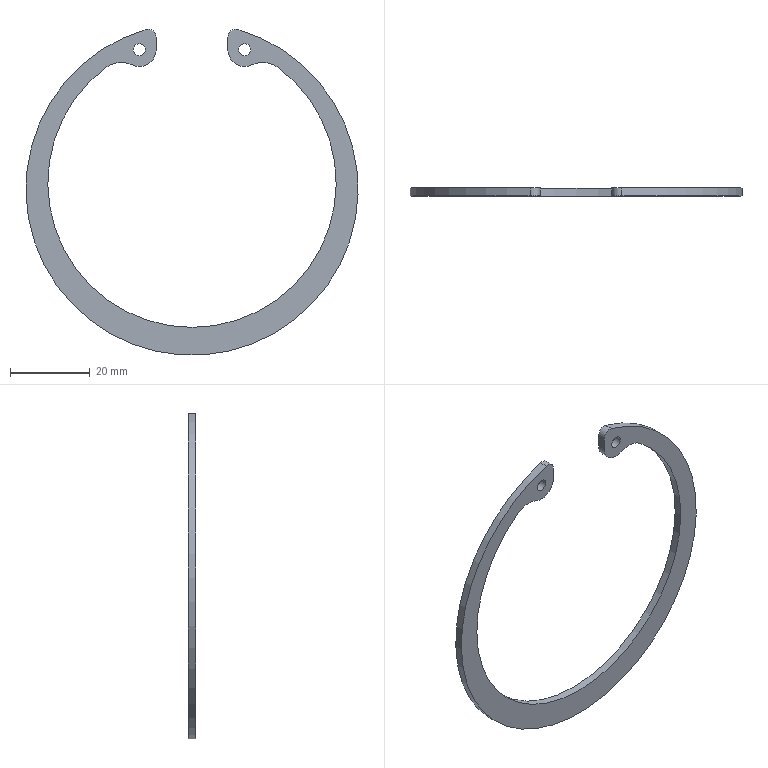Part | STEP file | Ring A80.65Г GOST 13943-86 | 1 solid | 14 faces | box 83.5 x 2 x 81.948 mm | volume 2646 mm3 | cylinder 10 | plane 4 | commonest cylinder face diameters 3 x2 4 x2 8.5 x2 13 x2 72.5 x1 83.5 x1
STEP:
#1=CARTESIAN_POINT('',(-21.685,0.,29.049));
#2=VERTEX_POINT('',#1);
#3=CARTESIAN_POINT('',(-21.685,2.,29.049));
#4=VERTEX_POINT('',#3);
#5=CARTESIAN_POINT('',(-21.685,0.,29.049));
#6=DIRECTION('',(0.,1.,0.));
#7=VECTOR('',#6,1.);
#8=LINE('',#5,#7);
#9=EDGE_CURVE('',#2,#4,#8,.T.);
#10=ORIENTED_EDGE('',*,*,#9,.F.);
#11=CARTESIAN_POINT('',(21.685,0.,29.049));
#12=VERTEX_POINT('',#11);
#13=CARTESIAN_POINT('',(0.,0.,0.));
#14=DIRECTION('',(0.,1.,0.));
#15=DIRECTION('',(0.5982,0.,0.8013));
#16=AXIS2_PLACEMENT_3D('',#13,#14,#15);
#17=CIRCLE('',#16,36.25);
#18=EDGE_CURVE('',#12,#2,#17,.T.);
#19=ORIENTED_EDGE('',*,*,#18,.F.);
#20=CARTESIAN_POINT('',(21.685,2.,29.049));
#21=VERTEX_POINT('',#20);
#22=CARTESIAN_POINT('',(21.685,0.,29.049));
#23=DIRECTION('',(0.,1.,0.));
#24=VECTOR('',#23,1.);
#25=LINE('',#22,#24);
#26=EDGE_CURVE('',#12,#21,#25,.T.);
#27=ORIENTED_EDGE('',*,*,#26,.T.);
#28=CARTESIAN_POINT('',(0.,2.,0.));
#29=DIRECTION('',(0.,1.,0.));
#30=DIRECTION('',(0.5982,0.,0.8013));
#31=AXIS2_PLACEMENT_3D('',#28,#29,#30);
#32=CIRCLE('',#31,36.25);
#33=EDGE_CURVE('',#4,#21,#32,.F.);
#34=ORIENTED_EDGE('',*,*,#33,.F.);
#35=EDGE_LOOP('',(#10,#19,#27,#34));
#36=FACE_BOUND('',#35,.T.);
#37=CARTESIAN_POINT('',(0.,0.,0.));
#38=DIRECTION('',(0.,1.,0.));
#39=DIRECTION('',(0.,0.,-1.));
#40=AXIS2_PLACEMENT_3D('',#37,#38,#39);
#41=CYLINDRICAL_SURFACE('',#40,36.25);
#42=ADVANCED_FACE('',(#36),#41,.F.);
#43=CARTESIAN_POINT('',(11.553,2.,38.62));
#44=VERTEX_POINT('',#43);
#45=CARTESIAN_POINT('',(11.553,0.,38.62));
#46=VERTEX_POINT('',#45);
#47=CARTESIAN_POINT('',(11.553,0.,38.62));
#48=DIRECTION('',(0.,1.,0.));
#49=VECTOR('',#48,1.);
#50=LINE('',#47,#49);
#51=EDGE_CURVE('',#44,#46,#50,.F.);
#52=ORIENTED_EDGE('',*,*,#51,.T.);
#53=CARTESIAN_POINT('',(-11.553,0.,38.62));
#54=VERTEX_POINT('',#53);
#55=CARTESIAN_POINT('',(0.,0.,-1.5));
#56=DIRECTION('',(0.,1.,0.));
#57=DIRECTION('',(0.2767,0.,0.9609));
#58=AXIS2_PLACEMENT_3D('',#55,#56,#57);
#59=CIRCLE('',#58,41.75);
#60=EDGE_CURVE('',#46,#54,#59,.T.);
#61=ORIENTED_EDGE('',*,*,#60,.T.);
#62=CARTESIAN_POINT('',(-11.553,2.,38.62));
#63=VERTEX_POINT('',#62);
#64=CARTESIAN_POINT('',(-11.553,0.,38.62));
#65=DIRECTION('',(0.,1.,0.));
#66=VECTOR('',#65,1.);
#67=LINE('',#64,#66);
#68=EDGE_CURVE('',#54,#63,#67,.T.);
#69=ORIENTED_EDGE('',*,*,#68,.T.);
#70=CARTESIAN_POINT('',(0.,2.,-1.5));
#71=DIRECTION('',(0.,1.,0.));
#72=DIRECTION('',(0.2767,0.,0.9609));
#73=AXIS2_PLACEMENT_3D('',#70,#71,#72);
#74=CIRCLE('',#73,41.75);
#75=EDGE_CURVE('',#44,#63,#74,.T.);
#76=ORIENTED_EDGE('',*,*,#75,.F.);
#77=EDGE_LOOP('',(#52,#61,#69,#76));
#78=FACE_BOUND('',#77,.T.);
#79=CARTESIAN_POINT('',(0.,0.,-1.5));
#80=DIRECTION('',(0.,1.,0.));
#81=DIRECTION('',(1.,0.,0.));
#82=AXIS2_PLACEMENT_3D('',#79,#80,#81);
#83=CYLINDRICAL_SURFACE('',#82,41.75);
#84=ADVANCED_FACE('',(#78),#83,.T.);
#85=CARTESIAN_POINT('',(9.,2.,36.698));
#86=VERTEX_POINT('',#85);
#87=CARTESIAN_POINT('',(11.,2.,36.698));
#88=DIRECTION('',(0.,-1.,0.));
#89=DIRECTION('',(0.2767,0.,0.9609));
#90=AXIS2_PLACEMENT_3D('',#87,#88,#89);
#91=CIRCLE('',#90,2.);
#92=EDGE_CURVE('',#44,#86,#91,.T.);
#93=ORIENTED_EDGE('',*,*,#92,.F.);
#94=ORIENTED_EDGE('',*,*,#75,.T.);
#95=CARTESIAN_POINT('',(-9.,2.,36.698));
#96=VERTEX_POINT('',#95);
#97=CARTESIAN_POINT('',(-11.,2.,36.698));
#98=DIRECTION('',(0.,-1.,0.));
#99=DIRECTION('',(1.,0.,0.));
#100=AXIS2_PLACEMENT_3D('',#97,#98,#99);
#101=CIRCLE('',#100,2.);
#102=EDGE_CURVE('',#96,#63,#101,.T.);
#103=ORIENTED_EDGE('',*,*,#102,.F.);
#104=CARTESIAN_POINT('',(-9.,2.,33.581));
#105=VERTEX_POINT('',#104);
#106=CARTESIAN_POINT('',(-9.,2.,33.581));
#107=DIRECTION('',(0.,0.,1.));
#108=VECTOR('',#107,1.);
#109=LINE('',#106,#108);
#110=EDGE_CURVE('',#96,#105,#109,.F.);
#111=ORIENTED_EDGE('',*,*,#110,.T.);
#112=CARTESIAN_POINT('',(-15.047,2.,29.73));
#113=VERTEX_POINT('',#112);
#114=CARTESIAN_POINT('',(-13.25,2.,33.581));
#115=DIRECTION('',(0.,-1.,0.));
#116=DIRECTION('',(-0.4229,0.,-0.9062));
#117=AXIS2_PLACEMENT_3D('',#114,#115,#116);
#118=CIRCLE('',#117,4.25);
#119=EDGE_CURVE('',#105,#113,#118,.F.);
#120=ORIENTED_EDGE('',*,*,#119,.T.);
#121=CARTESIAN_POINT('',(-17.797,2.,23.84));
#122=DIRECTION('',(0.,1.,0.));
#123=DIRECTION('',(-0.5982,0.,0.8013));
#124=AXIS2_PLACEMENT_3D('',#121,#122,#123);
#125=CIRCLE('',#124,6.5);
#126=EDGE_CURVE('',#113,#4,#125,.F.);
#127=ORIENTED_EDGE('',*,*,#126,.T.);
#128=ORIENTED_EDGE('',*,*,#33,.T.);
#129=CARTESIAN_POINT('',(15.047,2.,29.73));
#130=VERTEX_POINT('',#129);
#131=CARTESIAN_POINT('',(17.797,2.,23.84));
#132=DIRECTION('',(0.,1.,0.));
#133=DIRECTION('',(-0.4229,0.,0.9062));
#134=AXIS2_PLACEMENT_3D('',#131,#132,#133);
#135=CIRCLE('',#134,6.5);
#136=EDGE_CURVE('',#21,#130,#135,.F.);
#137=ORIENTED_EDGE('',*,*,#136,.T.);
#138=CARTESIAN_POINT('',(9.,2.,33.581));
#139=VERTEX_POINT('',#138);
#140=CARTESIAN_POINT('',(13.25,2.,33.581));
#141=DIRECTION('',(0.,-1.,0.));
#142=DIRECTION('',(-1.,0.,0.));
#143=AXIS2_PLACEMENT_3D('',#140,#141,#142);
#144=CIRCLE('',#143,4.25);
#145=EDGE_CURVE('',#130,#139,#144,.F.);
#146=ORIENTED_EDGE('',*,*,#145,.T.);
#147=CARTESIAN_POINT('',(9.,2.,36.698));
#148=DIRECTION('',(0.,0.,-1.));
#149=VECTOR('',#148,1.);
#150=LINE('',#147,#149);
#151=EDGE_CURVE('',#139,#86,#150,.F.);
#152=ORIENTED_EDGE('',*,*,#151,.T.);
#153=EDGE_LOOP('',(#93,#94,#103,#111,#120,#127,#128,#137,#146,#152));
#154=FACE_BOUND('',#153,.T.);
#155=CARTESIAN_POINT('',(-11.75,2.,33.581));
#156=VERTEX_POINT('',#155);
#157=CARTESIAN_POINT('',(-13.25,2.,33.581));
#158=DIRECTION('',(0.,1.,0.));
#159=DIRECTION('',(1.,0.,0.));
#160=AXIS2_PLACEMENT_3D('',#157,#158,#159);
#161=CIRCLE('',#160,1.5);
#162=EDGE_CURVE('',#156,#156,#161,.F.);
#163=ORIENTED_EDGE('',*,*,#162,.T.);
#164=EDGE_LOOP('',(#163));
#165=FACE_BOUND('',#164,.T.);
#166=CARTESIAN_POINT('',(11.75,2.,33.581));
#167=VERTEX_POINT('',#166);
#168=CARTESIAN_POINT('',(13.25,2.,33.581));
#169=DIRECTION('',(0.,1.,0.));
#170=DIRECTION('',(-1.,0.,0.));
#171=AXIS2_PLACEMENT_3D('',#168,#169,#170);
#172=CIRCLE('',#171,1.5);
#173=EDGE_CURVE('',#167,#167,#172,.F.);
#174=ORIENTED_EDGE('',*,*,#173,.T.);
#175=EDGE_LOOP('',(#174));
#176=FACE_BOUND('',#175,.T.);
#177=CARTESIAN_POINT('',(0.,2.,0.));
#178=DIRECTION('',(0.,1.,0.));
#179=DIRECTION('',(1.,0.,0.));
#180=AXIS2_PLACEMENT_3D('',#177,#178,#179);
#181=PLANE('',#180);
#182=ADVANCED_FACE('',(#154,#165,#176),#181,.T.);
#183=CARTESIAN_POINT('',(9.,0.,36.698));
#184=VERTEX_POINT('',#183);
#185=CARTESIAN_POINT('',(11.,0.,36.698));
#186=DIRECTION('',(0.,-1.,0.));
#187=DIRECTION('',(0.2767,0.,0.9609));
#188=AXIS2_PLACEMENT_3D('',#185,#186,#187);
#189=CIRCLE('',#188,2.);
#190=EDGE_CURVE('',#184,#46,#189,.F.);
#191=ORIENTED_EDGE('',*,*,#190,.F.);
#192=CARTESIAN_POINT('',(9.,0.,33.581));
#193=VERTEX_POINT('',#192);
#194=CARTESIAN_POINT('',(9.,0.,36.698));
#195=DIRECTION('',(0.,0.,-1.));
#196=VECTOR('',#195,1.);
#197=LINE('',#194,#196);
#198=EDGE_CURVE('',#184,#193,#197,.T.);
#199=ORIENTED_EDGE('',*,*,#198,.T.);
#200=CARTESIAN_POINT('',(15.047,0.,29.73));
#201=VERTEX_POINT('',#200);
#202=CARTESIAN_POINT('',(13.25,0.,33.581));
#203=DIRECTION('',(0.,-1.,0.));
#204=DIRECTION('',(-1.,0.,0.));
#205=AXIS2_PLACEMENT_3D('',#202,#203,#204);
#206=CIRCLE('',#205,4.25);
#207=EDGE_CURVE('',#193,#201,#206,.T.);
#208=ORIENTED_EDGE('',*,*,#207,.T.);
#209=CARTESIAN_POINT('',(17.797,0.,23.84));
#210=DIRECTION('',(0.,1.,0.));
#211=DIRECTION('',(-0.4229,0.,0.9062));
#212=AXIS2_PLACEMENT_3D('',#209,#210,#211);
#213=CIRCLE('',#212,6.5);
#214=EDGE_CURVE('',#201,#12,#213,.T.);
#215=ORIENTED_EDGE('',*,*,#214,.T.);
#216=ORIENTED_EDGE('',*,*,#18,.T.);
#217=CARTESIAN_POINT('',(-15.047,0.,29.73));
#218=VERTEX_POINT('',#217);
#219=CARTESIAN_POINT('',(-17.797,0.,23.84));
#220=DIRECTION('',(0.,1.,0.));
#221=DIRECTION('',(-0.5982,0.,0.8013));
#222=AXIS2_PLACEMENT_3D('',#219,#220,#221);
#223=CIRCLE('',#222,6.5);
#224=EDGE_CURVE('',#2,#218,#223,.T.);
#225=ORIENTED_EDGE('',*,*,#224,.T.);
#226=CARTESIAN_POINT('',(-9.,0.,33.581));
#227=VERTEX_POINT('',#226);
#228=CARTESIAN_POINT('',(-13.25,0.,33.581));
#229=DIRECTION('',(0.,-1.,0.));
#230=DIRECTION('',(-0.4229,0.,-0.9062));
#231=AXIS2_PLACEMENT_3D('',#228,#229,#230);
#232=CIRCLE('',#231,4.25);
#233=EDGE_CURVE('',#218,#227,#232,.T.);
#234=ORIENTED_EDGE('',*,*,#233,.T.);
#235=CARTESIAN_POINT('',(-9.,0.,36.698));
#236=VERTEX_POINT('',#235);
#237=CARTESIAN_POINT('',(-9.,0.,33.581));
#238=DIRECTION('',(0.,0.,1.));
#239=VECTOR('',#238,1.);
#240=LINE('',#237,#239);
#241=EDGE_CURVE('',#227,#236,#240,.T.);
#242=ORIENTED_EDGE('',*,*,#241,.T.);
#243=CARTESIAN_POINT('',(-11.,0.,36.698));
#244=DIRECTION('',(0.,-1.,0.));
#245=DIRECTION('',(1.,0.,0.));
#246=AXIS2_PLACEMENT_3D('',#243,#244,#245);
#247=CIRCLE('',#246,2.);
#248=EDGE_CURVE('',#54,#236,#247,.F.);
#249=ORIENTED_EDGE('',*,*,#248,.F.);
#250=ORIENTED_EDGE('',*,*,#60,.F.);
#251=EDGE_LOOP('',(#191,#199,#208,#215,#216,#225,#234,#242,#249,#250));
#252=FACE_BOUND('',#251,.T.);
#253=CARTESIAN_POINT('',(-11.75,0.,33.581));
#254=VERTEX_POINT('',#253);
#255=CARTESIAN_POINT('',(-13.25,0.,33.581));
#256=DIRECTION('',(0.,1.,0.));
#257=DIRECTION('',(1.,0.,0.));
#258=AXIS2_PLACEMENT_3D('',#255,#256,#257);
#259=CIRCLE('',#258,1.5);
#260=EDGE_CURVE('',#254,#254,#259,.T.);
#261=ORIENTED_EDGE('',*,*,#260,.T.);
#262=EDGE_LOOP('',(#261));
#263=FACE_BOUND('',#262,.T.);
#264=CARTESIAN_POINT('',(11.75,0.,33.581));
#265=VERTEX_POINT('',#264);
#266=CARTESIAN_POINT('',(13.25,0.,33.581));
#267=DIRECTION('',(0.,1.,0.));
#268=DIRECTION('',(-1.,0.,0.));
#269=AXIS2_PLACEMENT_3D('',#266,#267,#268);
#270=CIRCLE('',#269,1.5);
#271=EDGE_CURVE('',#265,#265,#270,.T.);
#272=ORIENTED_EDGE('',*,*,#271,.T.);
#273=EDGE_LOOP('',(#272));
#274=FACE_BOUND('',#273,.T.);
#275=CARTESIAN_POINT('',(0.,0.,0.));
#276=DIRECTION('',(0.,1.,0.));
#277=DIRECTION('',(1.,0.,0.));
#278=AXIS2_PLACEMENT_3D('',#275,#276,#277);
#279=PLANE('',#278);
#280=ADVANCED_FACE('',(#252,#263,#274),#279,.F.);
#281=ORIENTED_EDGE('',*,*,#173,.F.);
#282=EDGE_LOOP('',(#281));
#283=FACE_OUTER_BOUND('',#282,.T.);
#284=ORIENTED_EDGE('',*,*,#271,.F.);
#285=EDGE_LOOP('',(#284));
#286=FACE_OUTER_BOUND('',#285,.T.);
#287=CARTESIAN_POINT('',(13.25,0.,33.581));
#288=DIRECTION('',(0.,1.,0.));
#289=DIRECTION('',(-1.,0.,0.));
#290=AXIS2_PLACEMENT_3D('',#287,#288,#289);
#291=CYLINDRICAL_SURFACE('',#290,1.5);
#292=ADVANCED_FACE('',(#283,#286),#291,.F.);
#293=ORIENTED_EDGE('',*,*,#214,.F.);
#294=CARTESIAN_POINT('',(15.047,0.,29.73));
#295=DIRECTION('',(0.,1.,0.));
#296=VECTOR('',#295,1.);
#297=LINE('',#294,#296);
#298=EDGE_CURVE('',#201,#130,#297,.T.);
#299=ORIENTED_EDGE('',*,*,#298,.T.);
#300=ORIENTED_EDGE('',*,*,#136,.F.);
#301=ORIENTED_EDGE('',*,*,#26,.F.);
#302=EDGE_LOOP('',(#293,#299,#300,#301));
#303=FACE_BOUND('',#302,.T.);
#304=CARTESIAN_POINT('',(17.797,0.,23.84));
#305=DIRECTION('',(0.,1.,0.));
#306=DIRECTION('',(-0.4229,0.,0.9062));
#307=AXIS2_PLACEMENT_3D('',#304,#305,#306);
#308=CYLINDRICAL_SURFACE('',#307,6.5);
#309=ADVANCED_FACE('',(#303),#308,.F.);
#310=ORIENTED_EDGE('',*,*,#207,.F.);
#311=CARTESIAN_POINT('',(9.,0.,33.581));
#312=DIRECTION('',(0.,1.,0.));
#313=VECTOR('',#312,1.);
#314=LINE('',#311,#313);
#315=EDGE_CURVE('',#193,#139,#314,.T.);
#316=ORIENTED_EDGE('',*,*,#315,.T.);
#317=ORIENTED_EDGE('',*,*,#145,.F.);
#318=ORIENTED_EDGE('',*,*,#298,.F.);
#319=EDGE_LOOP('',(#310,#316,#317,#318));
#320=FACE_BOUND('',#319,.T.);
#321=CARTESIAN_POINT('',(13.25,0.,33.581));
#322=DIRECTION('',(0.,-1.,0.));
#323=DIRECTION('',(-1.,0.,0.));
#324=AXIS2_PLACEMENT_3D('',#321,#322,#323);
#325=CYLINDRICAL_SURFACE('',#324,4.25);
#326=ADVANCED_FACE('',(#320),#325,.T.);
#327=CARTESIAN_POINT('',(9.,0.,36.698));
#328=DIRECTION('',(0.,1.,0.));
#329=VECTOR('',#328,1.);
#330=LINE('',#327,#329);
#331=EDGE_CURVE('',#86,#184,#330,.F.);
#332=ORIENTED_EDGE('',*,*,#331,.F.);
#333=ORIENTED_EDGE('',*,*,#151,.F.);
#334=ORIENTED_EDGE('',*,*,#315,.F.);
#335=ORIENTED_EDGE('',*,*,#198,.F.);
#336=EDGE_LOOP('',(#332,#333,#334,#335));
#337=FACE_BOUND('',#336,.T.);
#338=CARTESIAN_POINT('',(9.,0.,83.5));
#339=DIRECTION('',(1.,0.,0.));
#340=DIRECTION('',(0.,0.,-1.));
#341=AXIS2_PLACEMENT_3D('',#338,#339,#340);
#342=PLANE('',#341);
#343=ADVANCED_FACE('',(#337),#342,.F.);
#344=ORIENTED_EDGE('',*,*,#126,.F.);
#345=CARTESIAN_POINT('',(-15.047,0.,29.73));
#346=DIRECTION('',(0.,1.,0.));
#347=VECTOR('',#346,1.);
#348=LINE('',#345,#347);
#349=EDGE_CURVE('',#218,#113,#348,.T.);
#350=ORIENTED_EDGE('',*,*,#349,.F.);
#351=ORIENTED_EDGE('',*,*,#224,.F.);
#352=ORIENTED_EDGE('',*,*,#9,.T.);
#353=EDGE_LOOP('',(#344,#350,#351,#352));
#354=FACE_BOUND('',#353,.T.);
#355=CARTESIAN_POINT('',(-17.797,0.,23.84));
#356=DIRECTION('',(0.,1.,0.));
#357=DIRECTION('',(-0.5982,0.,0.8013));
#358=AXIS2_PLACEMENT_3D('',#355,#356,#357);
#359=CYLINDRICAL_SURFACE('',#358,6.5);
#360=ADVANCED_FACE('',(#354),#359,.F.);
#361=ORIENTED_EDGE('',*,*,#68,.F.);
#362=ORIENTED_EDGE('',*,*,#248,.T.);
#363=CARTESIAN_POINT('',(-9.,0.,36.698));
#364=DIRECTION('',(0.,1.,0.));
#365=VECTOR('',#364,1.);
#366=LINE('',#363,#365);
#367=EDGE_CURVE('',#236,#96,#366,.T.);
#368=ORIENTED_EDGE('',*,*,#367,.T.);
#369=ORIENTED_EDGE('',*,*,#102,.T.);
#370=EDGE_LOOP('',(#361,#362,#368,#369));
#371=FACE_BOUND('',#370,.T.);
#372=CARTESIAN_POINT('',(-11.,-4.,36.698));
#373=DIRECTION('',(0.,-1.,0.));
#374=DIRECTION('',(1.,0.,0.));
#375=AXIS2_PLACEMENT_3D('',#372,#373,#374);
#376=CYLINDRICAL_SURFACE('',#375,2.);
#377=ADVANCED_FACE('',(#371),#376,.T.);
#378=ORIENTED_EDGE('',*,*,#367,.F.);
#379=ORIENTED_EDGE('',*,*,#241,.F.);
#380=CARTESIAN_POINT('',(-9.,0.,33.581));
#381=DIRECTION('',(0.,1.,0.));
#382=VECTOR('',#381,1.);
#383=LINE('',#380,#382);
#384=EDGE_CURVE('',#227,#105,#383,.T.);
#385=ORIENTED_EDGE('',*,*,#384,.T.);
#386=ORIENTED_EDGE('',*,*,#110,.F.);
#387=EDGE_LOOP('',(#378,#379,#385,#386));
#388=FACE_BOUND('',#387,.T.);
#389=CARTESIAN_POINT('',(-9.,0.,33.581));
#390=DIRECTION('',(-1.,0.,0.));
#391=DIRECTION('',(0.,0.,1.));
#392=AXIS2_PLACEMENT_3D('',#389,#390,#391);
#393=PLANE('',#392);
#394=ADVANCED_FACE('',(#388),#393,.F.);
#395=ORIENTED_EDGE('',*,*,#119,.F.);
#396=ORIENTED_EDGE('',*,*,#384,.F.);
#397=ORIENTED_EDGE('',*,*,#233,.F.);
#398=ORIENTED_EDGE('',*,*,#349,.T.);
#399=EDGE_LOOP('',(#395,#396,#397,#398));
#400=FACE_BOUND('',#399,.T.);
#401=CARTESIAN_POINT('',(-13.25,0.,33.581));
#402=DIRECTION('',(0.,-1.,0.));
#403=DIRECTION('',(-0.4229,0.,-0.9062));
#404=AXIS2_PLACEMENT_3D('',#401,#402,#403);
#405=CYLINDRICAL_SURFACE('',#404,4.25);
#406=ADVANCED_FACE('',(#400),#405,.T.);
#407=ORIENTED_EDGE('',*,*,#162,.F.);
#408=EDGE_LOOP('',(#407));
#409=FACE_OUTER_BOUND('',#408,.T.);
#410=ORIENTED_EDGE('',*,*,#260,.F.);
#411=EDGE_LOOP('',(#410));
#412=FACE_OUTER_BOUND('',#411,.T.);
#413=CARTESIAN_POINT('',(-13.25,0.,33.581));
#414=DIRECTION('',(0.,1.,0.));
#415=DIRECTION('',(1.,0.,0.));
#416=AXIS2_PLACEMENT_3D('',#413,#414,#415);
#417=CYLINDRICAL_SURFACE('',#416,1.5);
#418=ADVANCED_FACE('',(#409,#412),#417,.F.);
#419=ORIENTED_EDGE('',*,*,#51,.F.);
#420=ORIENTED_EDGE('',*,*,#92,.T.);
#421=ORIENTED_EDGE('',*,*,#331,.T.);
#422=ORIENTED_EDGE('',*,*,#190,.T.);
#423=EDGE_LOOP('',(#419,#420,#421,#422));
#424=FACE_BOUND('',#423,.T.);
#425=CARTESIAN_POINT('',(11.,-4.,36.698));
#426=DIRECTION('',(0.,1.,0.));
#427=DIRECTION('',(-1.,0.,0.));
#428=AXIS2_PLACEMENT_3D('',#425,#426,#427);
#429=CYLINDRICAL_SURFACE('',#428,2.);
#430=ADVANCED_FACE('',(#424),#429,.T.);
#431=CLOSED_SHELL('',(#42,#84,#182,#280,#292,#309,#326,#343,#360,#377,#394,#406,#418,#430));
#432=MANIFOLD_SOLID_BREP('',#431);
#433=(LENGTH_UNIT()NAMED_UNIT(*)SI_UNIT(.MILLI.,.METRE.));
#434=UNCERTAINTY_MEASURE_WITH_UNIT(LENGTH_MEASURE(0.00001),#433,'','');
#435=(NAMED_UNIT(*)PLANE_ANGLE_UNIT()SI_UNIT($,.RADIAN.));
#436=(NAMED_UNIT(*)SI_UNIT($,.STERADIAN.)SOLID_ANGLE_UNIT());
#437=(GEOMETRIC_REPRESENTATION_CONTEXT(3)GLOBAL_UNCERTAINTY_ASSIGNED_CONTEXT((#434))GLOBAL_UNIT_ASSIGNED_CONTEXT((#433,#435,#436))REPRESENTATION_CONTEXT('',''));
#438=ADVANCED_BREP_SHAPE_REPRESENTATION('',(#432),#437);